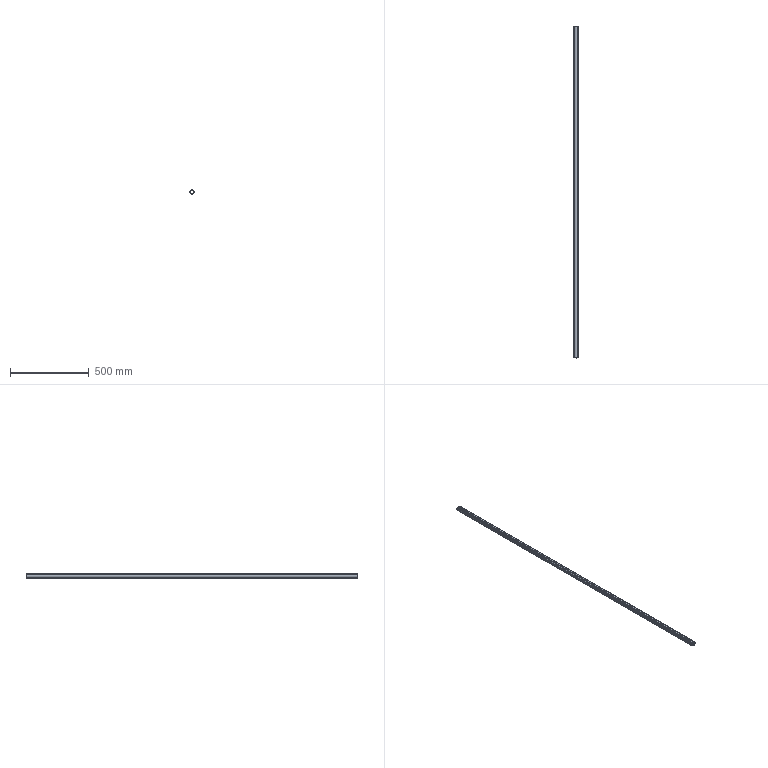Part | STEP file | FRONT GUIDE_ALUMINUM TUBE ITEM<As machined> | 1 solid | 52 faces | box 30 x 2110 x 30 mm | volume 421372 mm3 | cylinder 26 | plane 26 | commonest cylinder face diameters 24.6 x8 27 x5 30 x5 21 x4 25 x4